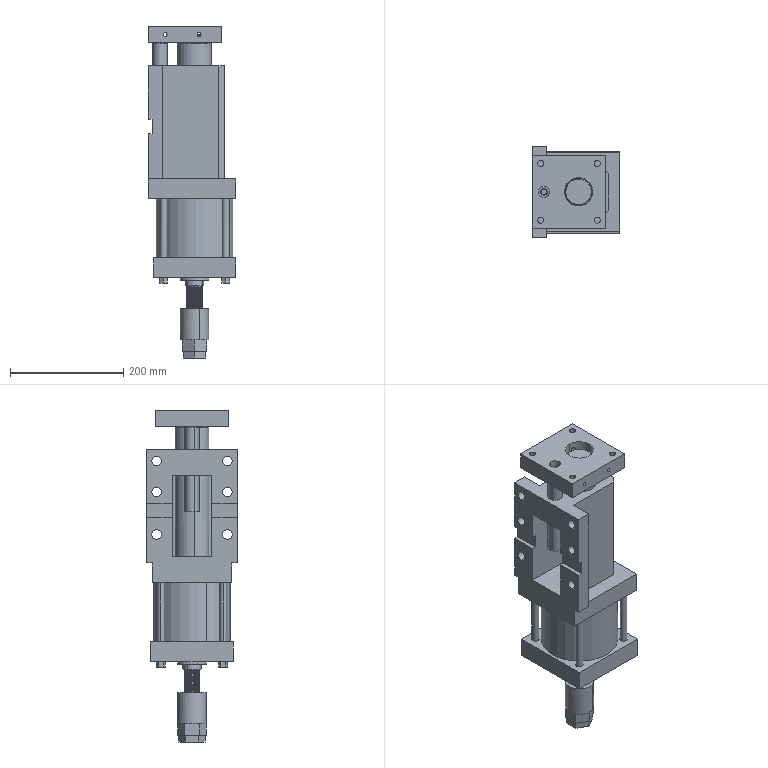Part | SolidWorks | features CompositeCurve 1 | 17 solids | 673 faces | box 155 x 160 x 586.3 mm | volume 4938149 mm3 | cylinder 415 | plane 170 | spline 45 | cone 43 | commonest cylinder face diameters 27 x109 12 x78 25 x26 19 x23 50 x18 39 x17